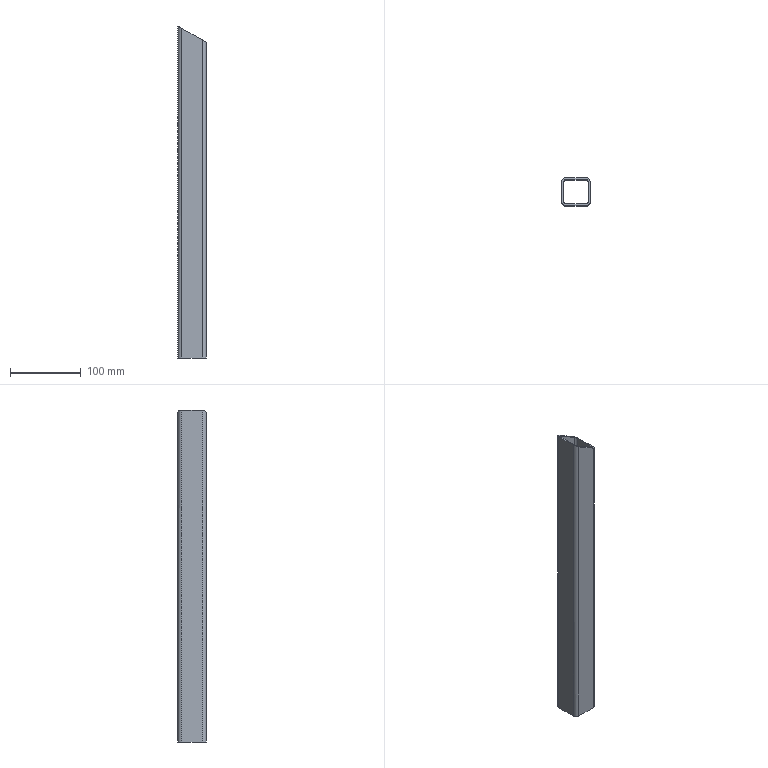Part | STEP file | DIN 59 410 - 40x40x2.9-500 | 1 solid | 18 faces | box 40 x 40 x 470 mm | volume 187371 mm3 | plane 10 | cylinder 8 | commonest cylinder face diameters 5.8 x4 11.6 x4